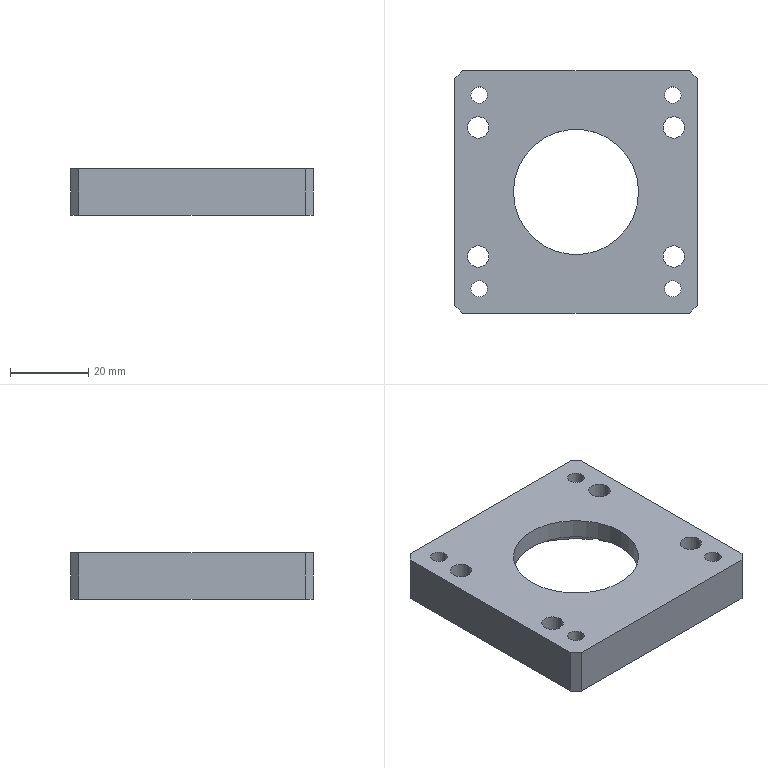Part | SolidWorks | features ICE 3, HoleWzd 2, Chamfer 1, Extrusion 1 | 1 solid | 53 faces | box 62 x 62 x 12 mm | volume 24839 mm3 | cylinder 36 | plane 17 | commonest cylinder face diameters 10.1 x12 4.2 x8 5.5 x8 32 x2 33.6 x2 38.4 x2